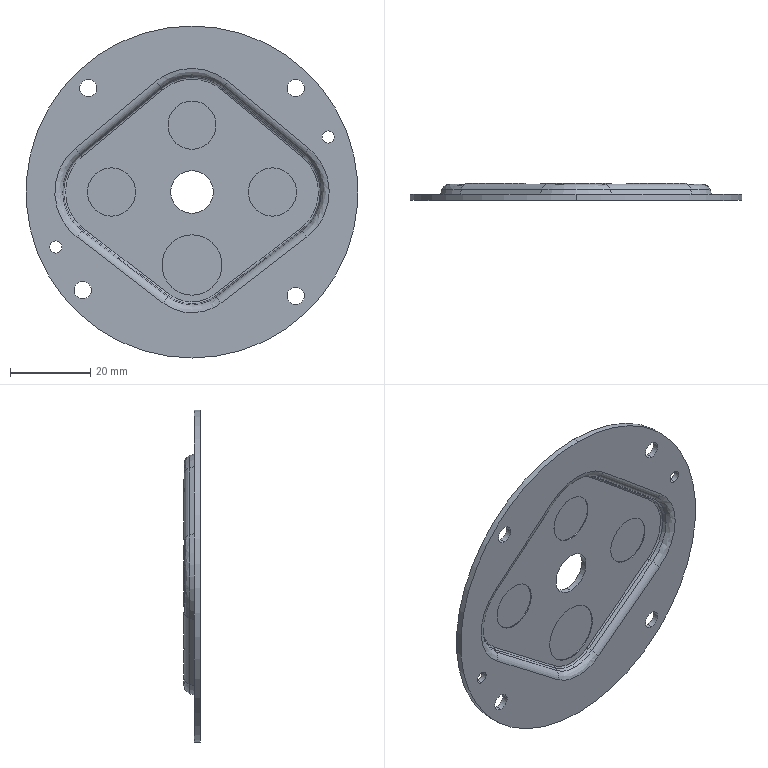Part | STEP file | 1 solid | 86 faces | box 82.5 x 4.2 x 82.5 mm | volume 8185 mm3 | cylinder 44 | plane 20 | spline 12 | cone 10 | commonest cylinder face diameters 4 x8 4.3 x8 15 x8 12 x6 1 x4 3 x4